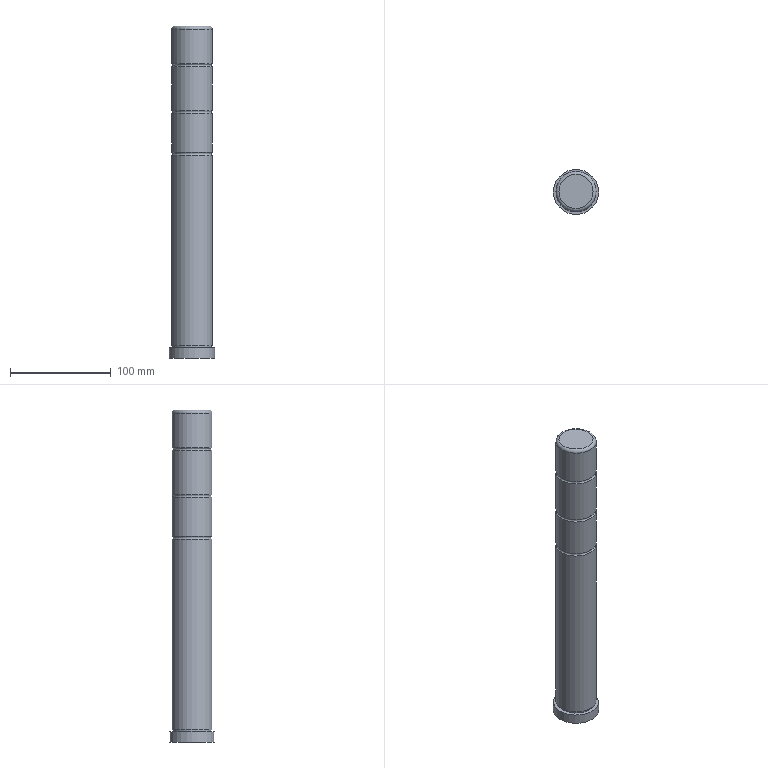Part | STEP file | 车灯-后视镜_id174_x_t | 1 solid | 14 faces | box 45 x 45 x 330 mm | volume 416787 mm3 | cylinder 6 | torus 4 | plane 4 | commonest cylinder face diameters 40 x4 38 x1 45 x1
STEP:
#1=CARTESIAN_POINT('',(-227.,232.,44.086));
#2=VERTEX_POINT('',#1);
#3=CARTESIAN_POINT('',(-207.,232.,44.086));
#4=DIRECTION('',(0.,0.,1.));
#5=DIRECTION('',(-1.,0.,0.));
#6=AXIS2_PLACEMENT_3D('',#3,#4,#5);
#7=CIRCLE('',#6,20.);
#8=EDGE_CURVE('',#2,#2,#7,.T.);
#9=ORIENTED_EDGE('',*,*,#8,.T.);
#10=EDGE_LOOP('',(#9));
#11=FACE_BOUND('',#10,.T.);
#12=CARTESIAN_POINT('',(-187.,232.,82.672));
#13=VERTEX_POINT('',#12);
#14=CARTESIAN_POINT('',(-207.,232.,82.672));
#15=DIRECTION('',(0.,0.,-1.));
#16=DIRECTION('',(1.,0.,0.));
#17=AXIS2_PLACEMENT_3D('',#14,#15,#16);
#18=CIRCLE('',#17,20.);
#19=EDGE_CURVE('',#13,#13,#18,.T.);
#20=ORIENTED_EDGE('',*,*,#19,.T.);
#21=EDGE_LOOP('',(#20));
#22=FACE_BOUND('',#21,.T.);
#23=CARTESIAN_POINT('',(-207.,232.,-90.5));
#24=DIRECTION('',(0.,0.,1.));
#25=DIRECTION('',(-1.,0.,0.));
#26=AXIS2_PLACEMENT_3D('',#23,#24,#25);
#27=CYLINDRICAL_SURFACE('',#26,20.);
#28=ADVANCED_FACE('',(#11,#22),#27,.T.);
#29=CARTESIAN_POINT('',(-227.,232.,85.5));
#30=VERTEX_POINT('',#29);
#31=CARTESIAN_POINT('',(-207.,232.,85.5));
#32=DIRECTION('',(0.,0.,1.));
#33=DIRECTION('',(-1.,0.,0.));
#34=AXIS2_PLACEMENT_3D('',#31,#32,#33);
#35=CIRCLE('',#34,20.);
#36=EDGE_CURVE('',#30,#30,#35,.T.);
#37=ORIENTED_EDGE('',*,*,#36,.T.);
#38=EDGE_LOOP('',(#37));
#39=FACE_BOUND('',#38,.T.);
#40=CARTESIAN_POINT('',(-187.,232.,129.086));
#41=VERTEX_POINT('',#40);
#42=CARTESIAN_POINT('',(-207.,232.,129.086));
#43=DIRECTION('',(0.,0.,-1.));
#44=DIRECTION('',(1.,0.,0.));
#45=AXIS2_PLACEMENT_3D('',#42,#43,#44);
#46=CIRCLE('',#45,20.);
#47=EDGE_CURVE('',#41,#41,#46,.T.);
#48=ORIENTED_EDGE('',*,*,#47,.T.);
#49=EDGE_LOOP('',(#48));
#50=FACE_BOUND('',#49,.T.);
#51=CARTESIAN_POINT('',(-207.,232.,-95.5));
#52=DIRECTION('',(0.,0.,1.));
#53=DIRECTION('',(-1.,0.,0.));
#54=AXIS2_PLACEMENT_3D('',#51,#52,#53);
#55=CYLINDRICAL_SURFACE('',#54,20.);
#56=ADVANCED_FACE('',(#39,#50),#55,.T.);
#57=CARTESIAN_POINT('',(-227.,232.,131.914));
#58=VERTEX_POINT('',#57);
#59=CARTESIAN_POINT('',(-207.,232.,131.914));
#60=DIRECTION('',(0.,0.,1.));
#61=DIRECTION('',(-1.,0.,0.));
#62=AXIS2_PLACEMENT_3D('',#59,#60,#61);
#63=CIRCLE('',#62,20.);
#64=EDGE_CURVE('',#58,#58,#63,.T.);
#65=ORIENTED_EDGE('',*,*,#64,.F.);
#66=EDGE_LOOP('',(#65));
#67=FACE_BOUND('',#66,.T.);
#68=ORIENTED_EDGE('',*,*,#47,.F.);
#69=EDGE_LOOP('',(#68));
#70=FACE_BOUND('',#69,.T.);
#71=CARTESIAN_POINT('',(-207.,232.,130.5));
#72=DIRECTION('',(0.,0.,1.));
#73=DIRECTION('',(-1.,0.,0.));
#74=AXIS2_PLACEMENT_3D('',#71,#72,#73);
#75=TOROIDAL_SURFACE('',#74,20.5,1.5);
#76=ADVANCED_FACE('',(#67,#70),#75,.F.);
#77=CARTESIAN_POINT('',(-224.,232.,169.5));
#78=VERTEX_POINT('',#77);
#79=CARTESIAN_POINT('',(-207.,232.,169.5));
#80=DIRECTION('',(0.,0.,-1.));
#81=DIRECTION('',(-1.,0.,0.));
#82=AXIS2_PLACEMENT_3D('',#79,#80,#81);
#83=CIRCLE('',#82,17.);
#84=EDGE_CURVE('',#78,#78,#83,.T.);
#85=ORIENTED_EDGE('',*,*,#84,.F.);
#86=EDGE_LOOP('',(#85));
#87=FACE_OUTER_BOUND('',#86,.T.);
#88=CARTESIAN_POINT('',(-207.,232.,169.5));
#89=DIRECTION('',(0.,0.,1.));
#90=DIRECTION('',(-1.,0.,0.));
#91=AXIS2_PLACEMENT_3D('',#88,#89,#90);
#92=PLANE('',#91);
#93=ADVANCED_FACE('',(#87),#92,.T.);
#94=ORIENTED_EDGE('',*,*,#84,.T.);
#95=EDGE_LOOP('',(#94));
#96=FACE_BOUND('',#95,.T.);
#97=CARTESIAN_POINT('',(-187.,232.,166.5));
#98=VERTEX_POINT('',#97);
#99=CARTESIAN_POINT('',(-207.,232.,166.5));
#100=DIRECTION('',(0.,0.,1.));
#101=DIRECTION('',(1.,0.,0.));
#102=AXIS2_PLACEMENT_3D('',#99,#100,#101);
#103=CIRCLE('',#102,20.);
#104=EDGE_CURVE('',#98,#98,#103,.T.);
#105=ORIENTED_EDGE('',*,*,#104,.T.);
#106=EDGE_LOOP('',(#105));
#107=FACE_BOUND('',#106,.T.);
#108=CARTESIAN_POINT('',(-207.,232.,166.5));
#109=DIRECTION('',(0.,0.,1.));
#110=DIRECTION('',(-1.,0.,0.));
#111=AXIS2_PLACEMENT_3D('',#108,#109,#110);
#112=TOROIDAL_SURFACE('',#111,17.,3.);
#113=ADVANCED_FACE('',(#96,#107),#112,.T.);
#114=ORIENTED_EDGE('',*,*,#64,.T.);
#115=EDGE_LOOP('',(#114));
#116=FACE_BOUND('',#115,.T.);
#117=ORIENTED_EDGE('',*,*,#104,.F.);
#118=EDGE_LOOP('',(#117));
#119=FACE_BOUND('',#118,.T.);
#120=CARTESIAN_POINT('',(-207.,232.,-20.5));
#121=DIRECTION('',(0.,0.,1.));
#122=DIRECTION('',(-1.,0.,0.));
#123=AXIS2_PLACEMENT_3D('',#120,#121,#122);
#124=CYLINDRICAL_SURFACE('',#123,20.);
#125=ADVANCED_FACE('',(#116,#119),#124,.T.);
#126=ORIENTED_EDGE('',*,*,#36,.F.);
#127=EDGE_LOOP('',(#126));
#128=FACE_BOUND('',#127,.T.);
#129=ORIENTED_EDGE('',*,*,#19,.F.);
#130=EDGE_LOOP('',(#129));
#131=FACE_BOUND('',#130,.T.);
#132=CARTESIAN_POINT('',(-207.,232.,84.086));
#133=DIRECTION('',(0.,0.,1.));
#134=DIRECTION('',(-1.,0.,0.));
#135=AXIS2_PLACEMENT_3D('',#132,#133,#134);
#136=TOROIDAL_SURFACE('',#135,20.5,1.5);
#137=ADVANCED_FACE('',(#128,#131),#136,.F.);
#138=ORIENTED_EDGE('',*,*,#8,.F.);
#139=EDGE_LOOP('',(#138));
#140=FACE_BOUND('',#139,.T.);
#141=CARTESIAN_POINT('',(-187.,232.,41.257));
#142=VERTEX_POINT('',#141);
#143=CARTESIAN_POINT('',(-207.,232.,41.257));
#144=DIRECTION('',(0.,0.,-1.));
#145=DIRECTION('',(1.,0.,0.));
#146=AXIS2_PLACEMENT_3D('',#143,#144,#145);
#147=CIRCLE('',#146,20.);
#148=EDGE_CURVE('',#142,#142,#147,.T.);
#149=ORIENTED_EDGE('',*,*,#148,.F.);
#150=EDGE_LOOP('',(#149));
#151=FACE_BOUND('',#150,.T.);
#152=CARTESIAN_POINT('',(-207.,232.,42.672));
#153=DIRECTION('',(0.,0.,1.));
#154=DIRECTION('',(-1.,0.,0.));
#155=AXIS2_PLACEMENT_3D('',#152,#153,#154);
#156=TOROIDAL_SURFACE('',#155,20.5,1.5);
#157=ADVANCED_FACE('',(#140,#151),#156,.F.);
#158=CARTESIAN_POINT('',(-227.,232.,-148.5));
#159=VERTEX_POINT('',#158);
#160=CARTESIAN_POINT('',(-207.,232.,-148.5));
#161=DIRECTION('',(0.,0.,1.));
#162=DIRECTION('',(-1.,0.,0.));
#163=AXIS2_PLACEMENT_3D('',#160,#161,#162);
#164=CIRCLE('',#163,20.);
#165=EDGE_CURVE('',#159,#159,#164,.T.);
#166=ORIENTED_EDGE('',*,*,#165,.T.);
#167=EDGE_LOOP('',(#166));
#168=FACE_BOUND('',#167,.T.);
#169=ORIENTED_EDGE('',*,*,#148,.T.);
#170=EDGE_LOOP('',(#169));
#171=FACE_BOUND('',#170,.T.);
#172=CARTESIAN_POINT('',(-207.,232.,-220.5));
#173=DIRECTION('',(0.,0.,1.));
#174=DIRECTION('',(-1.,0.,0.));
#175=AXIS2_PLACEMENT_3D('',#172,#173,#174);
#176=CYLINDRICAL_SURFACE('',#175,20.);
#177=ADVANCED_FACE('',(#168,#171),#176,.T.);
#178=CARTESIAN_POINT('',(-226.,232.,-148.5));
#179=VERTEX_POINT('',#178);
#180=CARTESIAN_POINT('',(-207.,232.,-148.5));
#181=DIRECTION('',(0.,0.,-1.));
#182=DIRECTION('',(-1.,0.,0.));
#183=AXIS2_PLACEMENT_3D('',#180,#181,#182);
#184=CIRCLE('',#183,19.);
#185=EDGE_CURVE('',#179,#179,#184,.T.);
#186=ORIENTED_EDGE('',*,*,#185,.T.);
#187=EDGE_LOOP('',(#186));
#188=FACE_BOUND('',#187,.T.);
#189=CARTESIAN_POINT('',(-226.,232.,-150.5));
#190=VERTEX_POINT('',#189);
#191=CARTESIAN_POINT('',(-207.,232.,-150.5));
#192=DIRECTION('',(0.,0.,-1.));
#193=DIRECTION('',(-1.,0.,0.));
#194=AXIS2_PLACEMENT_3D('',#191,#192,#193);
#195=CIRCLE('',#194,19.);
#196=EDGE_CURVE('',#190,#190,#195,.T.);
#197=ORIENTED_EDGE('',*,*,#196,.F.);
#198=EDGE_LOOP('',(#197));
#199=FACE_BOUND('',#198,.T.);
#200=CARTESIAN_POINT('',(-207.,232.,-149.5));
#201=DIRECTION('',(0.,0.,1.));
#202=DIRECTION('',(-1.,0.,0.));
#203=AXIS2_PLACEMENT_3D('',#200,#201,#202);
#204=CYLINDRICAL_SURFACE('',#203,19.);
#205=ADVANCED_FACE('',(#188,#199),#204,.T.);
#206=ORIENTED_EDGE('',*,*,#165,.F.);
#207=EDGE_LOOP('',(#206));
#208=FACE_BOUND('',#207,.T.);
#209=ORIENTED_EDGE('',*,*,#185,.F.);
#210=EDGE_LOOP('',(#209));
#211=FACE_BOUND('',#210,.T.);
#212=CARTESIAN_POINT('',(-207.,232.,-148.5));
#213=DIRECTION('',(0.,0.,1.));
#214=DIRECTION('',(-1.,0.,0.));
#215=AXIS2_PLACEMENT_3D('',#212,#213,#214);
#216=PLANE('',#215);
#217=ADVANCED_FACE('',(#208,#211),#216,.F.);
#218=CARTESIAN_POINT('',(-229.5,232.,-160.5));
#219=VERTEX_POINT('',#218);
#220=CARTESIAN_POINT('',(-207.,232.,-160.5));
#221=DIRECTION('',(0.,0.,-1.));
#222=DIRECTION('',(-1.,0.,0.));
#223=AXIS2_PLACEMENT_3D('',#220,#221,#222);
#224=CIRCLE('',#223,22.5);
#225=EDGE_CURVE('',#219,#219,#224,.T.);
#226=ORIENTED_EDGE('',*,*,#225,.T.);
#227=EDGE_LOOP('',(#226));
#228=FACE_OUTER_BOUND('',#227,.T.);
#229=CARTESIAN_POINT('',(-207.,232.,-160.5));
#230=DIRECTION('',(0.,0.,-1.));
#231=DIRECTION('',(1.,0.,0.));
#232=AXIS2_PLACEMENT_3D('',#229,#230,#231);
#233=PLANE('',#232);
#234=ADVANCED_FACE('',(#228),#233,.T.);
#235=CARTESIAN_POINT('',(-184.5,232.,-150.5));
#236=VERTEX_POINT('',#235);
#237=CARTESIAN_POINT('',(-207.,232.,-150.5));
#238=DIRECTION('',(0.,0.,1.));
#239=DIRECTION('',(1.,0.,0.));
#240=AXIS2_PLACEMENT_3D('',#237,#238,#239);
#241=CIRCLE('',#240,22.5);
#242=EDGE_CURVE('',#236,#236,#241,.T.);
#243=ORIENTED_EDGE('',*,*,#242,.F.);
#244=EDGE_LOOP('',(#243));
#245=FACE_BOUND('',#244,.T.);
#246=ORIENTED_EDGE('',*,*,#225,.F.);
#247=EDGE_LOOP('',(#246));
#248=FACE_BOUND('',#247,.T.);
#249=CARTESIAN_POINT('',(-207.,232.,-160.5));
#250=DIRECTION('',(0.,0.,1.));
#251=DIRECTION('',(-1.,0.,0.));
#252=AXIS2_PLACEMENT_3D('',#249,#250,#251);
#253=CYLINDRICAL_SURFACE('',#252,22.5);
#254=ADVANCED_FACE('',(#245,#248),#253,.T.);
#255=ORIENTED_EDGE('',*,*,#242,.T.);
#256=EDGE_LOOP('',(#255));
#257=FACE_BOUND('',#256,.T.);
#258=ORIENTED_EDGE('',*,*,#196,.T.);
#259=EDGE_LOOP('',(#258));
#260=FACE_BOUND('',#259,.T.);
#261=CARTESIAN_POINT('',(-207.,232.,-150.5));
#262=DIRECTION('',(0.,0.,1.));
#263=DIRECTION('',(-1.,0.,0.));
#264=AXIS2_PLACEMENT_3D('',#261,#262,#263);
#265=PLANE('',#264);
#266=ADVANCED_FACE('',(#257,#260),#265,.T.);
#267=CLOSED_SHELL('',(#28,#56,#76,#93,#113,#125,#137,#157,#177,#205,#217,#234,#254,#266));
#268=MANIFOLD_SOLID_BREP('',#267);
#269=(LENGTH_UNIT()NAMED_UNIT(*)SI_UNIT(.MILLI.,.METRE.));
#270=UNCERTAINTY_MEASURE_WITH_UNIT(LENGTH_MEASURE(0.00002),#269,'','');
#271=(NAMED_UNIT(*)PLANE_ANGLE_UNIT()SI_UNIT($,.RADIAN.));
#272=PLANE_ANGLE_MEASURE_WITH_UNIT(PLANE_ANGLE_MEASURE(0.01745),#271);
#273=DIMENSIONAL_EXPONENTS(0.,0.,0.,0.,0.,0.,0.);
#274=(CONVERSION_BASED_UNIT('DEGREE',#272)NAMED_UNIT(#273)PLANE_ANGLE_UNIT());
#275=(NAMED_UNIT(*)SI_UNIT($,.STERADIAN.)SOLID_ANGLE_UNIT());
#276=(GEOMETRIC_REPRESENTATION_CONTEXT(3)GLOBAL_UNCERTAINTY_ASSIGNED_CONTEXT((#270))GLOBAL_UNIT_ASSIGNED_CONTEXT((#269,#274,#275))REPRESENTATION_CONTEXT('',''));
#277=ADVANCED_BREP_SHAPE_REPRESENTATION('',(#268),#276);